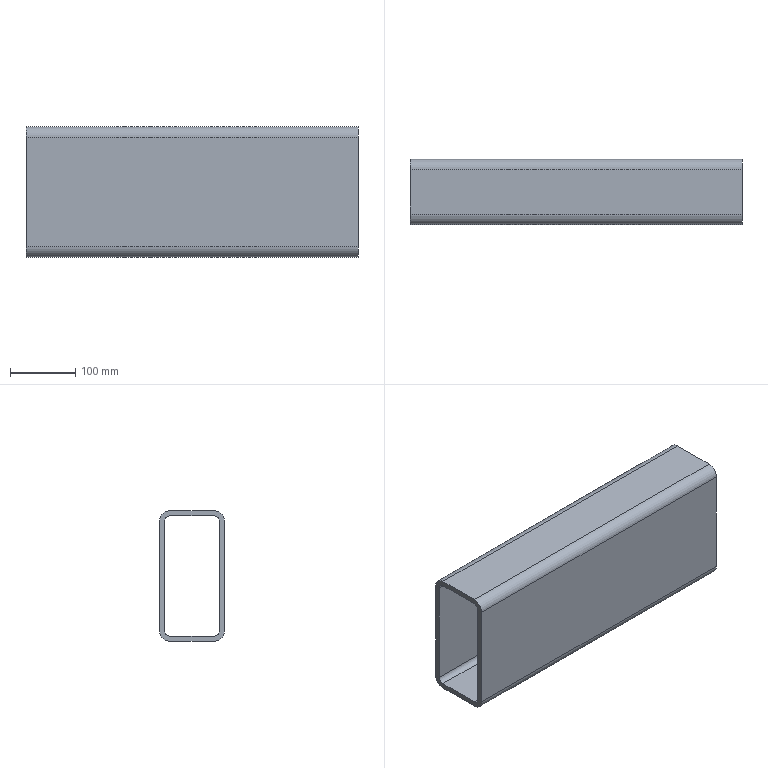Part | STEP file | 05-Longitudinal beam (flat tube 200x100x8)_default<machining> | 1 solid | 18 faces | box 509 x 100 x 200 mm | volume 2229006 mm3 | plane 10 | cylinder 8 | commonest cylinder face diameters 16 x4 32 x4
STEP:
#1=CARTESIAN_POINT('',(0.,0.,0.));
#2=DIRECTION('',(0.,0.,1.));
#3=DIRECTION('',(1.,0.,0.));
#4=AXIS2_PLACEMENT_3D('',#1,#2,#3);
#5=CARTESIAN_POINT('',(0.,50.,84.));
#6=VERTEX_POINT('',#5);
#7=CARTESIAN_POINT('',(0.,34.,100.));
#8=VERTEX_POINT('',#7);
#9=CARTESIAN_POINT('',(0.,34.,84.));
#10=DIRECTION('',(1.,0.,0.));
#11=DIRECTION('',(0.,0.,-1.));
#12=AXIS2_PLACEMENT_3D('',#9,#10,#11);
#13=CIRCLE('',#12,16.);
#14=CARTESIAN_POINT('',(509.,34.,84.));
#15=DIRECTION('',(-1.,0.,0.));
#16=DIRECTION('',(0.,0.,1.));
#17=AXIS2_PLACEMENT_3D('',#14,#15,#16);
#18=CYLINDRICAL_SURFACE('',#17,16.);
#19=CARTESIAN_POINT('',(3.142,509.));
#20=DIRECTION('',(-1.,0.));
#21=VECTOR('',#20,1.);
#22=LINE('',#19,#21);
#23=(GEOMETRIC_REPRESENTATION_CONTEXT(2)PARAMETRIC_REPRESENTATION_CONTEXT()REPRESENTATION_CONTEXT('',''));
#24=DEFINITIONAL_REPRESENTATION('',(#22),#23);
#25=PCURVE('',#18,#24);
#26=CARTESIAN_POINT('',(0.,34.,84.));
#27=DIRECTION('',(1.,0.,0.));
#28=DIRECTION('',(0.,0.,-1.));
#29=AXIS2_PLACEMENT_3D('',#26,#27,#28);
#30=PLANE('',#29);
#31=CARTESIAN_POINT('',(0.,0.));
#32=DIRECTION('',(1.,0.));
#33=AXIS2_PLACEMENT_2D('',#31,#32);
#34=CIRCLE('',#33,16.);
#35=(GEOMETRIC_REPRESENTATION_CONTEXT(2)PARAMETRIC_REPRESENTATION_CONTEXT()REPRESENTATION_CONTEXT('',''));
#36=DEFINITIONAL_REPRESENTATION('',(#34),#35);
#37=PCURVE('',#30,#36);
#38=SURFACE_CURVE('',#13,(#25,#37),.PCURVE_S1.);
#39=EDGE_CURVE('',#6,#8,#38,.T.);
#40=ORIENTED_EDGE('',*,*,#39,.T.);
#41=CARTESIAN_POINT('',(509.,34.,100.));
#42=VERTEX_POINT('',#41);
#43=CARTESIAN_POINT('',(509.,34.,100.));
#44=DIRECTION('',(-1.,0.,0.));
#45=VECTOR('',#44,1.);
#46=LINE('',#43,#45);
#47=CARTESIAN_POINT('',(0.,0.));
#48=DIRECTION('',(0.,1.));
#49=VECTOR('',#48,1.);
#50=LINE('',#47,#49);
#51=(GEOMETRIC_REPRESENTATION_CONTEXT(2)PARAMETRIC_REPRESENTATION_CONTEXT()REPRESENTATION_CONTEXT('',''));
#52=DEFINITIONAL_REPRESENTATION('',(#50),#51);
#53=PCURVE('',#18,#52);
#54=CARTESIAN_POINT('',(509.,34.,100.));
#55=DIRECTION('',(0.,0.,-1.));
#56=DIRECTION('',(-1.,0.,0.));
#57=AXIS2_PLACEMENT_3D('',#54,#55,#56);
#58=PLANE('',#57);
#59=CARTESIAN_POINT('',(0.,0.));
#60=DIRECTION('',(1.,0.));
#61=VECTOR('',#60,1.);
#62=LINE('',#59,#61);
#63=(GEOMETRIC_REPRESENTATION_CONTEXT(2)PARAMETRIC_REPRESENTATION_CONTEXT()REPRESENTATION_CONTEXT('',''));
#64=DEFINITIONAL_REPRESENTATION('',(#62),#63);
#65=PCURVE('',#58,#64);
#66=SURFACE_CURVE('',#46,(#53,#65),.PCURVE_S1.);
#67=EDGE_CURVE('',#42,#8,#66,.T.);
#68=ORIENTED_EDGE('',*,*,#67,.F.);
#69=CARTESIAN_POINT('',(509.,50.,84.));
#70=VERTEX_POINT('',#69);
#71=CARTESIAN_POINT('',(509.,34.,84.));
#72=DIRECTION('',(1.,0.,0.));
#73=DIRECTION('',(0.,0.,-1.));
#74=AXIS2_PLACEMENT_3D('',#71,#72,#73);
#75=CIRCLE('',#74,16.);
#76=CARTESIAN_POINT('',(3.142,0.));
#77=DIRECTION('',(-1.,0.));
#78=VECTOR('',#77,1.);
#79=LINE('',#76,#78);
#80=(GEOMETRIC_REPRESENTATION_CONTEXT(2)PARAMETRIC_REPRESENTATION_CONTEXT()REPRESENTATION_CONTEXT('',''));
#81=DEFINITIONAL_REPRESENTATION('',(#79),#80);
#82=PCURVE('',#18,#81);
#83=CARTESIAN_POINT('',(509.,34.,84.));
#84=DIRECTION('',(1.,0.,0.));
#85=DIRECTION('',(0.,0.,-1.));
#86=AXIS2_PLACEMENT_3D('',#83,#84,#85);
#87=PLANE('',#86);
#88=CARTESIAN_POINT('',(0.,0.));
#89=DIRECTION('',(1.,0.));
#90=AXIS2_PLACEMENT_2D('',#88,#89);
#91=CIRCLE('',#90,16.);
#92=(GEOMETRIC_REPRESENTATION_CONTEXT(2)PARAMETRIC_REPRESENTATION_CONTEXT()REPRESENTATION_CONTEXT('',''));
#93=DEFINITIONAL_REPRESENTATION('',(#91),#92);
#94=PCURVE('',#87,#93);
#95=SURFACE_CURVE('',#75,(#82,#94),.PCURVE_S1.);
#96=EDGE_CURVE('',#70,#42,#95,.T.);
#97=ORIENTED_EDGE('',*,*,#96,.F.);
#98=CARTESIAN_POINT('',(509.,50.,84.));
#99=DIRECTION('',(-1.,0.,0.));
#100=VECTOR('',#99,1.);
#101=LINE('',#98,#100);
#102=CARTESIAN_POINT('',(1.571,0.));
#103=DIRECTION('',(0.,1.));
#104=VECTOR('',#103,1.);
#105=LINE('',#102,#104);
#106=(GEOMETRIC_REPRESENTATION_CONTEXT(2)PARAMETRIC_REPRESENTATION_CONTEXT()REPRESENTATION_CONTEXT('',''));
#107=DEFINITIONAL_REPRESENTATION('',(#105),#106);
#108=PCURVE('',#18,#107);
#109=CARTESIAN_POINT('',(509.,50.,84.));
#110=DIRECTION('',(0.,-1.,0.));
#111=DIRECTION('',(0.,0.,-1.));
#112=AXIS2_PLACEMENT_3D('',#109,#110,#111);
#113=PLANE('',#112);
#114=CARTESIAN_POINT('',(0.,0.));
#115=DIRECTION('',(0.,-1.));
#116=VECTOR('',#115,1.);
#117=LINE('',#114,#116);
#118=(GEOMETRIC_REPRESENTATION_CONTEXT(2)PARAMETRIC_REPRESENTATION_CONTEXT()REPRESENTATION_CONTEXT('',''));
#119=DEFINITIONAL_REPRESENTATION('',(#117),#118);
#120=PCURVE('',#113,#119);
#121=SURFACE_CURVE('',#101,(#108,#120),.PCURVE_S1.);
#122=EDGE_CURVE('',#70,#6,#121,.T.);
#123=ORIENTED_EDGE('',*,*,#122,.T.);
#124=EDGE_LOOP('',(#40,#68,#97,#123));
#125=FACE_BOUND('',#124,.T.);
#126=ADVANCED_FACE('',(#125),#18,.T.);
#127=CARTESIAN_POINT('',(0.,-34.,100.));
#128=VERTEX_POINT('',#127);
#129=CARTESIAN_POINT('',(0.,34.,100.));
#130=DIRECTION('',(0.,-1.,0.));
#131=VECTOR('',#130,1.);
#132=LINE('',#129,#131);
#133=CARTESIAN_POINT('',(509.,0.));
#134=DIRECTION('',(0.,-1.));
#135=VECTOR('',#134,1.);
#136=LINE('',#133,#135);
#137=(GEOMETRIC_REPRESENTATION_CONTEXT(2)PARAMETRIC_REPRESENTATION_CONTEXT()REPRESENTATION_CONTEXT('',''));
#138=DEFINITIONAL_REPRESENTATION('',(#136),#137);
#139=PCURVE('',#58,#138);
#140=CARTESIAN_POINT('',(-16.,0.));
#141=DIRECTION('',(0.,-1.));
#142=VECTOR('',#141,1.);
#143=LINE('',#140,#142);
#144=(GEOMETRIC_REPRESENTATION_CONTEXT(2)PARAMETRIC_REPRESENTATION_CONTEXT()REPRESENTATION_CONTEXT('',''));
#145=DEFINITIONAL_REPRESENTATION('',(#143),#144);
#146=PCURVE('',#30,#145);
#147=SURFACE_CURVE('',#132,(#139,#146),.PCURVE_S1.);
#148=EDGE_CURVE('',#8,#128,#147,.T.);
#149=ORIENTED_EDGE('',*,*,#148,.T.);
#150=CARTESIAN_POINT('',(509.,-34.,100.));
#151=VERTEX_POINT('',#150);
#152=CARTESIAN_POINT('',(509.,-34.,100.));
#153=DIRECTION('',(-1.,0.,0.));
#154=VECTOR('',#153,1.);
#155=LINE('',#152,#154);
#156=CARTESIAN_POINT('',(0.,-68.));
#157=DIRECTION('',(1.,0.));
#158=VECTOR('',#157,1.);
#159=LINE('',#156,#158);
#160=(GEOMETRIC_REPRESENTATION_CONTEXT(2)PARAMETRIC_REPRESENTATION_CONTEXT()REPRESENTATION_CONTEXT('',''));
#161=DEFINITIONAL_REPRESENTATION('',(#159),#160);
#162=PCURVE('',#58,#161);
#163=CARTESIAN_POINT('',(509.,-34.,84.));
#164=DIRECTION('',(-1.,0.,0.));
#165=DIRECTION('',(0.,0.,1.));
#166=AXIS2_PLACEMENT_3D('',#163,#164,#165);
#167=CYLINDRICAL_SURFACE('',#166,16.);
#168=CARTESIAN_POINT('',(6.283,0.));
#169=DIRECTION('',(0.,1.));
#170=VECTOR('',#169,1.);
#171=LINE('',#168,#170);
#172=(GEOMETRIC_REPRESENTATION_CONTEXT(2)PARAMETRIC_REPRESENTATION_CONTEXT()REPRESENTATION_CONTEXT('',''));
#173=DEFINITIONAL_REPRESENTATION('',(#171),#172);
#174=PCURVE('',#167,#173);
#175=SURFACE_CURVE('',#155,(#162,#174),.PCURVE_S1.);
#176=EDGE_CURVE('',#151,#128,#175,.T.);
#177=ORIENTED_EDGE('',*,*,#176,.F.);
#178=CARTESIAN_POINT('',(509.,34.,100.));
#179=DIRECTION('',(0.,-1.,0.));
#180=VECTOR('',#179,1.);
#181=LINE('',#178,#180);
#182=CARTESIAN_POINT('',(0.,0.));
#183=DIRECTION('',(0.,-1.));
#184=VECTOR('',#183,1.);
#185=LINE('',#182,#184);
#186=(GEOMETRIC_REPRESENTATION_CONTEXT(2)PARAMETRIC_REPRESENTATION_CONTEXT()REPRESENTATION_CONTEXT('',''));
#187=DEFINITIONAL_REPRESENTATION('',(#185),#186);
#188=PCURVE('',#58,#187);
#189=CARTESIAN_POINT('',(-16.,0.));
#190=DIRECTION('',(0.,-1.));
#191=VECTOR('',#190,1.);
#192=LINE('',#189,#191);
#193=(GEOMETRIC_REPRESENTATION_CONTEXT(2)PARAMETRIC_REPRESENTATION_CONTEXT()REPRESENTATION_CONTEXT('',''));
#194=DEFINITIONAL_REPRESENTATION('',(#192),#193);
#195=PCURVE('',#87,#194);
#196=SURFACE_CURVE('',#181,(#188,#195),.PCURVE_S1.);
#197=EDGE_CURVE('',#42,#151,#196,.T.);
#198=ORIENTED_EDGE('',*,*,#197,.F.);
#199=ORIENTED_EDGE('',*,*,#67,.T.);
#200=EDGE_LOOP('',(#149,#177,#198,#199));
#201=FACE_BOUND('',#200,.T.);
#202=ADVANCED_FACE('',(#201),#58,.F.);
#203=CARTESIAN_POINT('',(0.,-50.,84.));
#204=VERTEX_POINT('',#203);
#205=CARTESIAN_POINT('',(0.,-34.,84.));
#206=DIRECTION('',(1.,0.,0.));
#207=DIRECTION('',(0.,0.,-1.));
#208=AXIS2_PLACEMENT_3D('',#205,#206,#207);
#209=CIRCLE('',#208,16.);
#210=CARTESIAN_POINT('',(9.425,509.));
#211=DIRECTION('',(-1.,0.));
#212=VECTOR('',#211,1.);
#213=LINE('',#210,#212);
#214=(GEOMETRIC_REPRESENTATION_CONTEXT(2)PARAMETRIC_REPRESENTATION_CONTEXT()REPRESENTATION_CONTEXT('',''));
#215=DEFINITIONAL_REPRESENTATION('',(#213),#214);
#216=PCURVE('',#167,#215);
#217=CARTESIAN_POINT('',(0.,-68.));
#218=DIRECTION('',(1.,0.));
#219=AXIS2_PLACEMENT_2D('',#217,#218);
#220=CIRCLE('',#219,16.);
#221=(GEOMETRIC_REPRESENTATION_CONTEXT(2)PARAMETRIC_REPRESENTATION_CONTEXT()REPRESENTATION_CONTEXT('',''));
#222=DEFINITIONAL_REPRESENTATION('',(#220),#221);
#223=PCURVE('',#30,#222);
#224=SURFACE_CURVE('',#209,(#216,#223),.PCURVE_S1.);
#225=EDGE_CURVE('',#128,#204,#224,.T.);
#226=ORIENTED_EDGE('',*,*,#225,.T.);
#227=CARTESIAN_POINT('',(509.,-50.,84.));
#228=VERTEX_POINT('',#227);
#229=CARTESIAN_POINT('',(509.,-50.,84.));
#230=DIRECTION('',(-1.,0.,0.));
#231=VECTOR('',#230,1.);
#232=LINE('',#229,#231);
#233=CARTESIAN_POINT('',(4.712,0.));
#234=DIRECTION('',(0.,1.));
#235=VECTOR('',#234,1.);
#236=LINE('',#233,#235);
#237=(GEOMETRIC_REPRESENTATION_CONTEXT(2)PARAMETRIC_REPRESENTATION_CONTEXT()REPRESENTATION_CONTEXT('',''));
#238=DEFINITIONAL_REPRESENTATION('',(#236),#237);
#239=PCURVE('',#167,#238);
#240=CARTESIAN_POINT('',(509.,-50.,-84.));
#241=DIRECTION('',(0.,1.,0.));
#242=DIRECTION('',(0.,0.,1.));
#243=AXIS2_PLACEMENT_3D('',#240,#241,#242);
#244=PLANE('',#243);
#245=CARTESIAN_POINT('',(168.,0.));
#246=DIRECTION('',(0.,-1.));
#247=VECTOR('',#246,1.);
#248=LINE('',#245,#247);
#249=(GEOMETRIC_REPRESENTATION_CONTEXT(2)PARAMETRIC_REPRESENTATION_CONTEXT()REPRESENTATION_CONTEXT('',''));
#250=DEFINITIONAL_REPRESENTATION('',(#248),#249);
#251=PCURVE('',#244,#250);
#252=SURFACE_CURVE('',#232,(#239,#251),.PCURVE_S1.);
#253=EDGE_CURVE('',#228,#204,#252,.T.);
#254=ORIENTED_EDGE('',*,*,#253,.F.);
#255=CARTESIAN_POINT('',(509.,-34.,84.));
#256=DIRECTION('',(1.,0.,0.));
#257=DIRECTION('',(0.,0.,-1.));
#258=AXIS2_PLACEMENT_3D('',#255,#256,#257);
#259=CIRCLE('',#258,16.);
#260=CARTESIAN_POINT('',(9.425,0.));
#261=DIRECTION('',(-1.,0.));
#262=VECTOR('',#261,1.);
#263=LINE('',#260,#262);
#264=(GEOMETRIC_REPRESENTATION_CONTEXT(2)PARAMETRIC_REPRESENTATION_CONTEXT()REPRESENTATION_CONTEXT('',''));
#265=DEFINITIONAL_REPRESENTATION('',(#263),#264);
#266=PCURVE('',#167,#265);
#267=CARTESIAN_POINT('',(0.,-68.));
#268=DIRECTION('',(1.,0.));
#269=AXIS2_PLACEMENT_2D('',#267,#268);
#270=CIRCLE('',#269,16.);
#271=(GEOMETRIC_REPRESENTATION_CONTEXT(2)PARAMETRIC_REPRESENTATION_CONTEXT()REPRESENTATION_CONTEXT('',''));
#272=DEFINITIONAL_REPRESENTATION('',(#270),#271);
#273=PCURVE('',#87,#272);
#274=SURFACE_CURVE('',#259,(#266,#273),.PCURVE_S1.);
#275=EDGE_CURVE('',#151,#228,#274,.T.);
#276=ORIENTED_EDGE('',*,*,#275,.F.);
#277=ORIENTED_EDGE('',*,*,#176,.T.);
#278=EDGE_LOOP('',(#226,#254,#276,#277));
#279=FACE_BOUND('',#278,.T.);
#280=ADVANCED_FACE('',(#279),#167,.T.);
#281=CARTESIAN_POINT('',(0.,-50.,-84.));
#282=VERTEX_POINT('',#281);
#283=CARTESIAN_POINT('',(0.,-50.,-84.));
#284=DIRECTION('',(0.,0.,-1.));
#285=VECTOR('',#284,1.);
#286=LINE('',#283,#285);
#287=CARTESIAN_POINT('',(0.,-509.));
#288=DIRECTION('',(-1.,0.));
#289=VECTOR('',#288,1.);
#290=LINE('',#287,#289);
#291=(GEOMETRIC_REPRESENTATION_CONTEXT(2)PARAMETRIC_REPRESENTATION_CONTEXT()REPRESENTATION_CONTEXT('',''));
#292=DEFINITIONAL_REPRESENTATION('',(#290),#291);
#293=PCURVE('',#244,#292);
#294=CARTESIAN_POINT('',(168.,-84.));
#295=DIRECTION('',(1.,0.));
#296=VECTOR('',#295,1.);
#297=LINE('',#294,#296);
#298=(GEOMETRIC_REPRESENTATION_CONTEXT(2)PARAMETRIC_REPRESENTATION_CONTEXT()REPRESENTATION_CONTEXT('',''));
#299=DEFINITIONAL_REPRESENTATION('',(#297),#298);
#300=PCURVE('',#30,#299);
#301=SURFACE_CURVE('',#286,(#293,#300),.PCURVE_S1.);
#302=EDGE_CURVE('',#204,#282,#301,.T.);
#303=ORIENTED_EDGE('',*,*,#302,.T.);
#304=CARTESIAN_POINT('',(509.,-50.,-84.));
#305=VERTEX_POINT('',#304);
#306=CARTESIAN_POINT('',(509.,-50.,-84.));
#307=DIRECTION('',(-1.,0.,0.));
#308=VECTOR('',#307,1.);
#309=LINE('',#306,#308);
#310=CARTESIAN_POINT('',(0.,0.));
#311=DIRECTION('',(0.,-1.));
#312=VECTOR('',#311,1.);
#313=LINE('',#310,#312);
#314=(GEOMETRIC_REPRESENTATION_CONTEXT(2)PARAMETRIC_REPRESENTATION_CONTEXT()REPRESENTATION_CONTEXT('',''));
#315=DEFINITIONAL_REPRESENTATION('',(#313),#314);
#316=PCURVE('',#244,#315);
#317=CARTESIAN_POINT('',(509.,-34.,-84.));
#318=DIRECTION('',(-1.,0.,0.));
#319=DIRECTION('',(0.,0.,1.));
#320=AXIS2_PLACEMENT_3D('',#317,#318,#319);
#321=CYLINDRICAL_SURFACE('',#320,16.);
#322=CARTESIAN_POINT('',(4.712,0.));
#323=DIRECTION('',(0.,1.));
#324=VECTOR('',#323,1.);
#325=LINE('',#322,#324);
#326=(GEOMETRIC_REPRESENTATION_CONTEXT(2)PARAMETRIC_REPRESENTATION_CONTEXT()REPRESENTATION_CONTEXT('',''));
#327=DEFINITIONAL_REPRESENTATION('',(#325),#326);
#328=PCURVE('',#321,#327);
#329=SURFACE_CURVE('',#309,(#316,#328),.PCURVE_S1.);
#330=EDGE_CURVE('',#305,#282,#329,.T.);
#331=ORIENTED_EDGE('',*,*,#330,.F.);
#332=CARTESIAN_POINT('',(509.,-50.,-84.));
#333=DIRECTION('',(0.,0.,-1.));
#334=VECTOR('',#333,1.);
#335=LINE('',#332,#334);
#336=CARTESIAN_POINT('',(0.,0.));
#337=DIRECTION('',(-1.,0.));
#338=VECTOR('',#337,1.);
#339=LINE('',#336,#338);
#340=(GEOMETRIC_REPRESENTATION_CONTEXT(2)PARAMETRIC_REPRESENTATION_CONTEXT()REPRESENTATION_CONTEXT('',''));
#341=DEFINITIONAL_REPRESENTATION('',(#339),#340);
#342=PCURVE('',#244,#341);
#343=CARTESIAN_POINT('',(168.,-84.));
#344=DIRECTION('',(1.,0.));
#345=VECTOR('',#344,1.);
#346=LINE('',#343,#345);
#347=(GEOMETRIC_REPRESENTATION_CONTEXT(2)PARAMETRIC_REPRESENTATION_CONTEXT()REPRESENTATION_CONTEXT('',''));
#348=DEFINITIONAL_REPRESENTATION('',(#346),#347);
#349=PCURVE('',#87,#348);
#350=SURFACE_CURVE('',#335,(#342,#349),.PCURVE_S1.);
#351=EDGE_CURVE('',#228,#305,#350,.T.);
#352=ORIENTED_EDGE('',*,*,#351,.F.);
#353=ORIENTED_EDGE('',*,*,#253,.T.);
#354=EDGE_LOOP('',(#303,#331,#352,#353));
#355=FACE_BOUND('',#354,.T.);
#356=ADVANCED_FACE('',(#355),#244,.F.);
#357=CARTESIAN_POINT('',(0.,-34.,-100.));
#358=VERTEX_POINT('',#357);
#359=CARTESIAN_POINT('',(0.,-34.,-84.));
#360=DIRECTION('',(1.,0.,0.));
#361=DIRECTION('',(0.,0.,-1.));
#362=AXIS2_PLACEMENT_3D('',#359,#360,#361);
#363=CIRCLE('',#362,16.);
#364=CARTESIAN_POINT('',(9.425,509.));
#365=DIRECTION('',(-1.,0.));
#366=VECTOR('',#365,1.);
#367=LINE('',#364,#366);
#368=(GEOMETRIC_REPRESENTATION_CONTEXT(2)PARAMETRIC_REPRESENTATION_CONTEXT()REPRESENTATION_CONTEXT('',''));
#369=DEFINITIONAL_REPRESENTATION('',(#367),#368);
#370=PCURVE('',#321,#369);
#371=CARTESIAN_POINT('',(168.,-68.));
#372=DIRECTION('',(1.,0.));
#373=AXIS2_PLACEMENT_2D('',#371,#372);
#374=CIRCLE('',#373,16.);
#375=(GEOMETRIC_REPRESENTATION_CONTEXT(2)PARAMETRIC_REPRESENTATION_CONTEXT()REPRESENTATION_CONTEXT('',''));
#376=DEFINITIONAL_REPRESENTATION('',(#374),#375);
#377=PCURVE('',#30,#376);
#378=SURFACE_CURVE('',#363,(#370,#377),.PCURVE_S1.);
#379=EDGE_CURVE('',#282,#358,#378,.T.);
#380=ORIENTED_EDGE('',*,*,#379,.T.);
#381=CARTESIAN_POINT('',(509.,-34.,-100.));
#382=VERTEX_POINT('',#381);
#383=CARTESIAN_POINT('',(509.,-34.,-100.));
#384=DIRECTION('',(-1.,0.,0.));
#385=VECTOR('',#384,1.);
#386=LINE('',#383,#385);
#387=CARTESIAN_POINT('',(3.142,0.));
#388=DIRECTION('',(0.,1.));
#389=VECTOR('',#388,1.);
#390=LINE('',#387,#389);
#391=(GEOMETRIC_REPRESENTATION_CONTEXT(2)PARAMETRIC_REPRESENTATION_CONTEXT()REPRESENTATION_CONTEXT('',''));
#392=DEFINITIONAL_REPRESENTATION('',(#390),#391);
#393=PCURVE('',#321,#392);
#394=CARTESIAN_POINT('',(509.,-34.,-100.));
#395=DIRECTION('',(0.,0.,1.));
#396=DIRECTION('',(1.,0.,0.));
#397=AXIS2_PLACEMENT_3D('',#394,#395,#396);
#398=PLANE('',#397);
#399=CARTESIAN_POINT('',(0.,0.));
#400=DIRECTION('',(-1.,0.));
#401=VECTOR('',#400,1.);
#402=LINE('',#399,#401);
#403=(GEOMETRIC_REPRESENTATION_CONTEXT(2)PARAMETRIC_REPRESENTATION_CONTEXT()REPRESENTATION_CONTEXT('',''));
#404=DEFINITIONAL_REPRESENTATION('',(#402),#403);
#405=PCURVE('',#398,#404);
#406=SURFACE_CURVE('',#386,(#393,#405),.PCURVE_S1.);
#407=EDGE_CURVE('',#382,#358,#406,.T.);
#408=ORIENTED_EDGE('',*,*,#407,.F.);
#409=CARTESIAN_POINT('',(509.,-34.,-84.));
#410=DIRECTION('',(1.,0.,0.));
#411=DIRECTION('',(0.,0.,-1.));
#412=AXIS2_PLACEMENT_3D('',#409,#410,#411);
#413=CIRCLE('',#412,16.);
#414=CARTESIAN_POINT('',(9.425,0.));
#415=DIRECTION('',(-1.,0.));
#416=VECTOR('',#415,1.);
#417=LINE('',#414,#416);
#418=(GEOMETRIC_REPRESENTATION_CONTEXT(2)PARAMETRIC_REPRESENTATION_CONTEXT()REPRESENTATION_CONTEXT('',''));
#419=DEFINITIONAL_REPRESENTATION('',(#417),#418);
#420=PCURVE('',#321,#419);
#421=CARTESIAN_POINT('',(168.,-68.));
#422=DIRECTION('',(1.,0.));
#423=AXIS2_PLACEMENT_2D('',#421,#422);
#424=CIRCLE('',#423,16.);
#425=(GEOMETRIC_REPRESENTATION_CONTEXT(2)PARAMETRIC_REPRESENTATION_CONTEXT()REPRESENTATION_CONTEXT('',''));
#426=DEFINITIONAL_REPRESENTATION('',(#424),#425);
#427=PCURVE('',#87,#426);
#428=SURFACE_CURVE('',#413,(#420,#427),.PCURVE_S1.);
#429=EDGE_CURVE('',#305,#382,#428,.T.);
#430=ORIENTED_EDGE('',*,*,#429,.F.);
#431=ORIENTED_EDGE('',*,*,#330,.T.);
#432=EDGE_LOOP('',(#380,#408,#430,#431));
#433=FACE_BOUND('',#432,.T.);
#434=ADVANCED_FACE('',(#433),#321,.T.);
#435=CARTESIAN_POINT('',(0.,34.,-100.));
#436=VERTEX_POINT('',#435);
#437=CARTESIAN_POINT('',(0.,-34.,-100.));
#438=DIRECTION('',(0.,1.,0.));
#439=VECTOR('',#438,1.);
#440=LINE('',#437,#439);
#441=CARTESIAN_POINT('',(-509.,0.));
#442=DIRECTION('',(0.,1.));
#443=VECTOR('',#442,1.);
#444=LINE('',#441,#443);
#445=(GEOMETRIC_REPRESENTATION_CONTEXT(2)PARAMETRIC_REPRESENTATION_CONTEXT()REPRESENTATION_CONTEXT('',''));
#446=DEFINITIONAL_REPRESENTATION('',(#444),#445);
#447=PCURVE('',#398,#446);
#448=CARTESIAN_POINT('',(184.,-68.));
#449=DIRECTION('',(0.,1.));
#450=VECTOR('',#449,1.);
#451=LINE('',#448,#450);
#452=(GEOMETRIC_REPRESENTATION_CONTEXT(2)PARAMETRIC_REPRESENTATION_CONTEXT()REPRESENTATION_CONTEXT('',''));
#453=DEFINITIONAL_REPRESENTATION('',(#451),#452);
#454=PCURVE('',#30,#453);
#455=SURFACE_CURVE('',#440,(#447,#454),.PCURVE_S1.);
#456=EDGE_CURVE('',#358,#436,#455,.T.);
#457=ORIENTED_EDGE('',*,*,#456,.T.);
#458=CARTESIAN_POINT('',(509.,34.,-100.));
#459=VERTEX_POINT('',#458);
#460=CARTESIAN_POINT('',(509.,34.,-100.));
#461=DIRECTION('',(-1.,0.,0.));
#462=VECTOR('',#461,1.);
#463=LINE('',#460,#462);
#464=CARTESIAN_POINT('',(0.,68.));
#465=DIRECTION('',(-1.,0.));
#466=VECTOR('',#465,1.);
#467=LINE('',#464,#466);
#468=(GEOMETRIC_REPRESENTATION_CONTEXT(2)PARAMETRIC_REPRESENTATION_CONTEXT()REPRESENTATION_CONTEXT('',''));
#469=DEFINITIONAL_REPRESENTATION('',(#467),#468);
#470=PCURVE('',#398,#469);
#471=CARTESIAN_POINT('',(509.,34.,-84.));
#472=DIRECTION('',(-1.,0.,0.));
#473=DIRECTION('',(0.,0.,1.));
#474=AXIS2_PLACEMENT_3D('',#471,#472,#473);
#475=CYLINDRICAL_SURFACE('',#474,16.);
#476=CARTESIAN_POINT('',(3.142,0.));
#477=DIRECTION('',(0.,1.));
#478=VECTOR('',#477,1.);
#479=LINE('',#476,#478);
#480=(GEOMETRIC_REPRESENTATION_CONTEXT(2)PARAMETRIC_REPRESENTATION_CONTEXT()REPRESENTATION_CONTEXT('',''));
#481=DEFINITIONAL_REPRESENTATION('',(#479),#480);
#482=PCURVE('',#475,#481);
#483=SURFACE_CURVE('',#463,(#470,#482),.PCURVE_S1.);
#484=EDGE_CURVE('',#459,#436,#483,.T.);
#485=ORIENTED_EDGE('',*,*,#484,.F.);
#486=CARTESIAN_POINT('',(509.,-34.,-100.));
#487=DIRECTION('',(0.,1.,0.));
#488=VECTOR('',#487,1.);
#489=LINE('',#486,#488);
#490=CARTESIAN_POINT('',(0.,0.));
#491=DIRECTION('',(0.,1.));
#492=VECTOR('',#491,1.);
#493=LINE('',#490,#492);
#494=(GEOMETRIC_REPRESENTATION_CONTEXT(2)PARAMETRIC_REPRESENTATION_CONTEXT()REPRESENTATION_CONTEXT('',''));
#495=DEFINITIONAL_REPRESENTATION('',(#493),#494);
#496=PCURVE('',#398,#495);
#497=CARTESIAN_POINT('',(184.,-68.));
#498=DIRECTION('',(0.,1.));
#499=VECTOR('',#498,1.);
#500=LINE('',#497,#499);
#501=(GEOMETRIC_REPRESENTATION_CONTEXT(2)PARAMETRIC_REPRESENTATION_CONTEXT()REPRESENTATION_CONTEXT('',''));
#502=DEFINITIONAL_REPRESENTATION('',(#500),#501);
#503=PCURVE('',#87,#502);
#504=SURFACE_CURVE('',#489,(#496,#503),.PCURVE_S1.);
#505=EDGE_CURVE('',#382,#459,#504,.T.);
#506=ORIENTED_EDGE('',*,*,#505,.F.);
#507=ORIENTED_EDGE('',*,*,#407,.T.);
#508=EDGE_LOOP('',(#457,#485,#506,#507));
#509=FACE_BOUND('',#508,.T.);
#510=ADVANCED_FACE('',(#509),#398,.F.);
#511=CARTESIAN_POINT('',(0.,50.,-84.));
#512=VERTEX_POINT('',#511);
#513=CARTESIAN_POINT('',(0.,34.,-84.));
#514=DIRECTION('',(1.,0.,0.));
#515=DIRECTION('',(0.,0.,-1.));
#516=AXIS2_PLACEMENT_3D('',#513,#514,#515);
#517=CIRCLE('',#516,16.);
#518=CARTESIAN_POINT('',(3.142,509.));
#519=DIRECTION('',(-1.,0.));
#520=VECTOR('',#519,1.);
#521=LINE('',#518,#520);
#522=(GEOMETRIC_REPRESENTATION_CONTEXT(2)PARAMETRIC_REPRESENTATION_CONTEXT()REPRESENTATION_CONTEXT('',''));
#523=DEFINITIONAL_REPRESENTATION('',(#521),#522);
#524=PCURVE('',#475,#523);
#525=CARTESIAN_POINT('',(168.,0.));
#526=DIRECTION('',(1.,0.));
#527=AXIS2_PLACEMENT_2D('',#525,#526);
#528=CIRCLE('',#527,16.);
#529=(GEOMETRIC_REPRESENTATION_CONTEXT(2)PARAMETRIC_REPRESENTATION_CONTEXT()REPRESENTATION_CONTEXT('',''));
#530=DEFINITIONAL_REPRESENTATION('',(#528),#529);
#531=PCURVE('',#30,#530);
#532=SURFACE_CURVE('',#517,(#524,#531),.PCURVE_S1.);
#533=EDGE_CURVE('',#436,#512,#532,.T.);
#534=ORIENTED_EDGE('',*,*,#533,.T.);
#535=CARTESIAN_POINT('',(509.,50.,-84.));
#536=VERTEX_POINT('',#535);
#537=CARTESIAN_POINT('',(509.,50.,-84.));
#538=DIRECTION('',(-1.,0.,0.));
#539=VECTOR('',#538,1.);
#540=LINE('',#537,#539);
#541=CARTESIAN_POINT('',(1.571,0.));
#542=DIRECTION('',(0.,1.));
#543=VECTOR('',#542,1.);
#544=LINE('',#541,#543);
#545=(GEOMETRIC_REPRESENTATION_CONTEXT(2)PARAMETRIC_REPRESENTATION_CONTEXT()REPRESENTATION_CONTEXT('',''));
#546=DEFINITIONAL_REPRESENTATION('',(#544),#545);
#547=PCURVE('',#475,#546);
#548=CARTESIAN_POINT('',(168.,0.));
#549=DIRECTION('',(0.,-1.));
#550=VECTOR('',#549,1.);
#551=LINE('',#548,#550);
#552=(GEOMETRIC_REPRESENTATION_CONTEXT(2)PARAMETRIC_REPRESENTATION_CONTEXT()REPRESENTATION_CONTEXT('',''));
#553=DEFINITIONAL_REPRESENTATION('',(#551),#552);
#554=PCURVE('',#113,#553);
#555=SURFACE_CURVE('',#540,(#547,#554),.PCURVE_S1.);
#556=EDGE_CURVE('',#536,#512,#555,.T.);
#557=ORIENTED_EDGE('',*,*,#556,.F.);
#558=CARTESIAN_POINT('',(509.,34.,-84.));
#559=DIRECTION('',(1.,0.,0.));
#560=DIRECTION('',(0.,0.,-1.));
#561=AXIS2_PLACEMENT_3D('',#558,#559,#560);
#562=CIRCLE('',#561,16.);
#563=CARTESIAN_POINT('',(3.142,0.));
#564=DIRECTION('',(-1.,0.));
#565=VECTOR('',#564,1.);
#566=LINE('',#563,#565);
#567=(GEOMETRIC_REPRESENTATION_CONTEXT(2)PARAMETRIC_REPRESENTATION_CONTEXT()REPRESENTATION_CONTEXT('',''));
#568=DEFINITIONAL_REPRESENTATION('',(#566),#567);
#569=PCURVE('',#475,#568);
#570=CARTESIAN_POINT('',(168.,0.));
#571=DIRECTION('',(1.,0.));
#572=AXIS2_PLACEMENT_2D('',#570,#571);
#573=CIRCLE('',#572,16.);
#574=(GEOMETRIC_REPRESENTATION_CONTEXT(2)PARAMETRIC_REPRESENTATION_CONTEXT()REPRESENTATION_CONTEXT('',''));
#575=DEFINITIONAL_REPRESENTATION('',(#573),#574);
#576=PCURVE('',#87,#575);
#577=SURFACE_CURVE('',#562,(#569,#576),.PCURVE_S1.);
#578=EDGE_CURVE('',#459,#536,#577,.T.);
#579=ORIENTED_EDGE('',*,*,#578,.F.);
#580=ORIENTED_EDGE('',*,*,#484,.T.);
#581=EDGE_LOOP('',(#534,#557,#579,#580));
#582=FACE_BOUND('',#581,.T.);
#583=ADVANCED_FACE('',(#582),#475,.T.);
#584=CARTESIAN_POINT('',(509.,-42.,84.));
#585=VERTEX_POINT('',#584);
#586=CARTESIAN_POINT('',(0.,-42.,84.));
#587=VERTEX_POINT('',#586);
#588=CARTESIAN_POINT('',(509.,-42.,84.));
#589=DIRECTION('',(-1.,0.,0.));
#590=VECTOR('',#589,1.);
#591=LINE('',#588,#590);
#592=CARTESIAN_POINT('',(509.,-34.,84.));
#593=DIRECTION('',(-1.,0.,0.));
#594=DIRECTION('',(0.,0.,1.));
#595=AXIS2_PLACEMENT_3D('',#592,#593,#594);
#596=CYLINDRICAL_SURFACE('',#595,8.);
#597=CARTESIAN_POINT('',(4.712,0.));
#598=DIRECTION('',(0.,1.));
#599=VECTOR('',#598,1.);
#600=LINE('',#597,#599);
#601=(GEOMETRIC_REPRESENTATION_CONTEXT(2)PARAMETRIC_REPRESENTATION_CONTEXT()REPRESENTATION_CONTEXT('',''));
#602=DEFINITIONAL_REPRESENTATION('',(#600),#601);
#603=PCURVE('',#596,#602);
#604=CARTESIAN_POINT('',(509.,-42.,-84.));
#605=DIRECTION('',(0.,1.,0.));
#606=DIRECTION('',(0.,0.,1.));
#607=AXIS2_PLACEMENT_3D('',#604,#605,#606);
#608=PLANE('',#607);
#609=CARTESIAN_POINT('',(168.,0.));
#610=DIRECTION('',(0.,-1.));
#611=VECTOR('',#610,1.);
#612=LINE('',#609,#611);
#613=(GEOMETRIC_REPRESENTATION_CONTEXT(2)PARAMETRIC_REPRESENTATION_CONTEXT()REPRESENTATION_CONTEXT('',''));
#614=DEFINITIONAL_REPRESENTATION('',(#612),#613);
#615=PCURVE('',#608,#614);
#616=SURFACE_CURVE('',#591,(#603,#615),.PCURVE_S1.);
#617=EDGE_CURVE('',#585,#587,#616,.T.);
#618=ORIENTED_EDGE('',*,*,#617,.F.);
#619=CARTESIAN_POINT('',(509.,-34.,92.));
#620=VERTEX_POINT('',#619);
#621=CARTESIAN_POINT('',(509.,-34.,84.));
#622=DIRECTION('',(1.,0.,0.));
#623=DIRECTION('',(0.,0.,-1.));
#624=AXIS2_PLACEMENT_3D('',#621,#622,#623);
#625=CIRCLE('',#624,8.);
#626=CARTESIAN_POINT('',(9.425,0.));
#627=DIRECTION('',(-1.,0.));
#628=VECTOR('',#627,1.);
#629=LINE('',#626,#628);
#630=(GEOMETRIC_REPRESENTATION_CONTEXT(2)PARAMETRIC_REPRESENTATION_CONTEXT()REPRESENTATION_CONTEXT('',''));
#631=DEFINITIONAL_REPRESENTATION('',(#629),#630);
#632=PCURVE('',#596,#631);
#633=CARTESIAN_POINT('',(0.,-68.));
#634=DIRECTION('',(1.,0.));
#635=AXIS2_PLACEMENT_2D('',#633,#634);
#636=CIRCLE('',#635,8.);
#637=(GEOMETRIC_REPRESENTATION_CONTEXT(2)PARAMETRIC_REPRESENTATION_CONTEXT()REPRESENTATION_CONTEXT('',''));
#638=DEFINITIONAL_REPRESENTATION('',(#636),#637);
#639=PCURVE('',#87,#638);
#640=SURFACE_CURVE('',#625,(#632,#639),.PCURVE_S1.);
#641=EDGE_CURVE('',#620,#585,#640,.T.);
#642=ORIENTED_EDGE('',*,*,#641,.F.);
#643=CARTESIAN_POINT('',(0.,-34.,92.));
#644=VERTEX_POINT('',#643);
#645=CARTESIAN_POINT('',(509.,-34.,92.));
#646=DIRECTION('',(-1.,0.,0.));
#647=VECTOR('',#646,1.);
#648=LINE('',#645,#647);
#649=CARTESIAN_POINT('',(6.283,0.));
#650=DIRECTION('',(0.,1.));
#651=VECTOR('',#650,1.);
#652=LINE('',#649,#651);
#653=(GEOMETRIC_REPRESENTATION_CONTEXT(2)PARAMETRIC_REPRESENTATION_CONTEXT()REPRESENTATION_CONTEXT('',''));
#654=DEFINITIONAL_REPRESENTATION('',(#652),#653);
#655=PCURVE('',#596,#654);
#656=CARTESIAN_POINT('',(509.,34.,92.));
#657=DIRECTION('',(0.,0.,-1.));
#658=DIRECTION('',(-1.,0.,0.));
#659=AXIS2_PLACEMENT_3D('',#656,#657,#658);
#660=PLANE('',#659);
#661=CARTESIAN_POINT('',(0.,-68.));
#662=DIRECTION('',(1.,0.));
#663=VECTOR('',#662,1.);
#664=LINE('',#661,#663);
#665=(GEOMETRIC_REPRESENTATION_CONTEXT(2)PARAMETRIC_REPRESENTATION_CONTEXT()REPRESENTATION_CONTEXT('',''));
#666=DEFINITIONAL_REPRESENTATION('',(#664),#665);
#667=PCURVE('',#660,#666);
#668=SURFACE_CURVE('',#648,(#655,#667),.PCURVE_S1.);
#669=EDGE_CURVE('',#620,#644,#668,.T.);
#670=ORIENTED_EDGE('',*,*,#669,.T.);
#671=CARTESIAN_POINT('',(0.,-34.,84.));
#672=DIRECTION('',(1.,0.,0.));
#673=DIRECTION('',(0.,0.,-1.));
#674=AXIS2_PLACEMENT_3D('',#671,#672,#673);
#675=CIRCLE('',#674,8.);
#676=CARTESIAN_POINT('',(9.425,509.));
#677=DIRECTION('',(-1.,0.));
#678=VECTOR('',#677,1.);
#679=LINE('',#676,#678);
#680=(GEOMETRIC_REPRESENTATION_CONTEXT(2)PARAMETRIC_REPRESENTATION_CONTEXT()REPRESENTATION_CONTEXT('',''));
#681=DEFINITIONAL_REPRESENTATION('',(#679),#680);
#682=PCURVE('',#596,#681);
#683=CARTESIAN_POINT('',(0.,-68.));
#684=DIRECTION('',(1.,0.));
#685=AXIS2_PLACEMENT_2D('',#683,#684);
#686=CIRCLE('',#685,8.);
#687=(GEOMETRIC_REPRESENTATION_CONTEXT(2)PARAMETRIC_REPRESENTATION_CONTEXT()REPRESENTATION_CONTEXT('',''));
#688=DEFINITIONAL_REPRESENTATION('',(#686),#687);
#689=PCURVE('',#30,#688);
#690=SURFACE_CURVE('',#675,(#682,#689),.PCURVE_S1.);
#691=EDGE_CURVE('',#644,#587,#690,.T.);
#692=ORIENTED_EDGE('',*,*,#691,.T.);
#693=EDGE_LOOP('',(#618,#642,#670,#692));
#694=FACE_BOUND('',#693,.F.);
#695=ADVANCED_FACE('',(#694),#596,.F.);
#696=CARTESIAN_POINT('',(0.,34.,92.));
#697=VERTEX_POINT('',#696);
#698=CARTESIAN_POINT('',(0.,34.,92.));
#699=DIRECTION('',(0.,-1.,0.));
#700=VECTOR('',#699,1.);
#701=LINE('',#698,#700);
#702=CARTESIAN_POINT('',(509.,0.));
#703=DIRECTION('',(0.,-1.));
#704=VECTOR('',#703,1.);
#705=LINE('',#702,#704);
#706=(GEOMETRIC_REPRESENTATION_CONTEXT(2)PARAMETRIC_REPRESENTATION_CONTEXT()REPRESENTATION_CONTEXT('',''));
#707=DEFINITIONAL_REPRESENTATION('',(#705),#706);
#708=PCURVE('',#660,#707);
#709=CARTESIAN_POINT('',(-8.,0.));
#710=DIRECTION('',(0.,-1.));
#711=VECTOR('',#710,1.);
#712=LINE('',#709,#711);
#713=(GEOMETRIC_REPRESENTATION_CONTEXT(2)PARAMETRIC_REPRESENTATION_CONTEXT()REPRESENTATION_CONTEXT('',''));
#714=DEFINITIONAL_REPRESENTATION('',(#712),#713);
#715=PCURVE('',#30,#714);
#716=SURFACE_CURVE('',#701,(#708,#715),.PCURVE_S1.);
#717=EDGE_CURVE('',#697,#644,#716,.T.);
#718=ORIENTED_EDGE('',*,*,#717,.F.);
#719=CARTESIAN_POINT('',(509.,34.,92.));
#720=VERTEX_POINT('',#719);
#721=CARTESIAN_POINT('',(509.,34.,92.));
#722=DIRECTION('',(-1.,0.,0.));
#723=VECTOR('',#722,1.);
#724=LINE('',#721,#723);
#725=CARTESIAN_POINT('',(0.,0.));
#726=DIRECTION('',(1.,0.));
#727=VECTOR('',#726,1.);
#728=LINE('',#725,#727);
#729=(GEOMETRIC_REPRESENTATION_CONTEXT(2)PARAMETRIC_REPRESENTATION_CONTEXT()REPRESENTATION_CONTEXT('',''));
#730=DEFINITIONAL_REPRESENTATION('',(#728),#729);
#731=PCURVE('',#660,#730);
#732=CARTESIAN_POINT('',(509.,34.,84.));
#733=DIRECTION('',(-1.,0.,0.));
#734=DIRECTION('',(0.,0.,1.));
#735=AXIS2_PLACEMENT_3D('',#732,#733,#734);
#736=CYLINDRICAL_SURFACE('',#735,8.);
#737=CARTESIAN_POINT('',(0.,0.));
#738=DIRECTION('',(0.,1.));
#739=VECTOR('',#738,1.);
#740=LINE('',#737,#739);
#741=(GEOMETRIC_REPRESENTATION_CONTEXT(2)PARAMETRIC_REPRESENTATION_CONTEXT()REPRESENTATION_CONTEXT('',''));
#742=DEFINITIONAL_REPRESENTATION('',(#740),#741);
#743=PCURVE('',#736,#742);
#744=SURFACE_CURVE('',#724,(#731,#743),.PCURVE_S1.);
#745=EDGE_CURVE('',#720,#697,#744,.T.);
#746=ORIENTED_EDGE('',*,*,#745,.F.);
#747=CARTESIAN_POINT('',(509.,34.,92.));
#748=DIRECTION('',(0.,-1.,0.));
#749=VECTOR('',#748,1.);
#750=LINE('',#747,#749);
#751=CARTESIAN_POINT('',(0.,0.));
#752=DIRECTION('',(0.,-1.));
#753=VECTOR('',#752,1.);
#754=LINE('',#751,#753);
#755=(GEOMETRIC_REPRESENTATION_CONTEXT(2)PARAMETRIC_REPRESENTATION_CONTEXT()REPRESENTATION_CONTEXT('',''));
#756=DEFINITIONAL_REPRESENTATION('',(#754),#755);
#757=PCURVE('',#660,#756);
#758=CARTESIAN_POINT('',(-8.,0.));
#759=DIRECTION('',(0.,-1.));
#760=VECTOR('',#759,1.);
#761=LINE('',#758,#760);
#762=(GEOMETRIC_REPRESENTATION_CONTEXT(2)PARAMETRIC_REPRESENTATION_CONTEXT()REPRESENTATION_CONTEXT('',''));
#763=DEFINITIONAL_REPRESENTATION('',(#761),#762);
#764=PCURVE('',#87,#763);
#765=SURFACE_CURVE('',#750,(#757,#764),.PCURVE_S1.);
#766=EDGE_CURVE('',#720,#620,#765,.T.);
#767=ORIENTED_EDGE('',*,*,#766,.T.);
#768=ORIENTED_EDGE('',*,*,#669,.T.);
#769=EDGE_LOOP('',(#718,#746,#767,#768));
#770=FACE_BOUND('',#769,.T.);
#771=ADVANCED_FACE('',(#770),#660,.T.);
#772=ORIENTED_EDGE('',*,*,#745,.F.);
#773=CARTESIAN_POINT('',(509.,42.,84.));
#774=VERTEX_POINT('',#773);
#775=CARTESIAN_POINT('',(509.,34.,84.));
#776=DIRECTION('',(1.,0.,0.));
#777=DIRECTION('',(0.,0.,-1.));
#778=AXIS2_PLACEMENT_3D('',#775,#776,#777);
#779=CIRCLE('',#778,8.);
#780=CARTESIAN_POINT('',(3.142,0.));
#781=DIRECTION('',(-1.,0.));
#782=VECTOR('',#781,1.);
#783=LINE('',#780,#782);
#784=(GEOMETRIC_REPRESENTATION_CONTEXT(2)PARAMETRIC_REPRESENTATION_CONTEXT()REPRESENTATION_CONTEXT('',''));
#785=DEFINITIONAL_REPRESENTATION('',(#783),#784);
#786=PCURVE('',#736,#785);
#787=CARTESIAN_POINT('',(0.,0.));
#788=DIRECTION('',(1.,0.));
#789=AXIS2_PLACEMENT_2D('',#787,#788);
#790=CIRCLE('',#789,8.);
#791=(GEOMETRIC_REPRESENTATION_CONTEXT(2)PARAMETRIC_REPRESENTATION_CONTEXT()REPRESENTATION_CONTEXT('',''));
#792=DEFINITIONAL_REPRESENTATION('',(#790),#791);
#793=PCURVE('',#87,#792);
#794=SURFACE_CURVE('',#779,(#786,#793),.PCURVE_S1.);
#795=EDGE_CURVE('',#774,#720,#794,.T.);
#796=ORIENTED_EDGE('',*,*,#795,.F.);
#797=CARTESIAN_POINT('',(0.,42.,84.));
#798=VERTEX_POINT('',#797);
#799=CARTESIAN_POINT('',(509.,42.,84.));
#800=DIRECTION('',(-1.,0.,0.));
#801=VECTOR('',#800,1.);
#802=LINE('',#799,#801);
#803=CARTESIAN_POINT('',(1.571,0.));
#804=DIRECTION('',(0.,1.));
#805=VECTOR('',#804,1.);
#806=LINE('',#803,#805);
#807=(GEOMETRIC_REPRESENTATION_CONTEXT(2)PARAMETRIC_REPRESENTATION_CONTEXT()REPRESENTATION_CONTEXT('',''));
#808=DEFINITIONAL_REPRESENTATION('',(#806),#807);
#809=PCURVE('',#736,#808);
#810=CARTESIAN_POINT('',(509.,42.,84.));
#811=DIRECTION('',(0.,-1.,0.));
#812=DIRECTION('',(0.,0.,-1.));
#813=AXIS2_PLACEMENT_3D('',#810,#811,#812);
#814=PLANE('',#813);
#815=CARTESIAN_POINT('',(0.,0.));
#816=DIRECTION('',(0.,-1.));
#817=VECTOR('',#816,1.);
#818=LINE('',#815,#817);
#819=(GEOMETRIC_REPRESENTATION_CONTEXT(2)PARAMETRIC_REPRESENTATION_CONTEXT()REPRESENTATION_CONTEXT('',''));
#820=DEFINITIONAL_REPRESENTATION('',(#818),#819);
#821=PCURVE('',#814,#820);
#822=SURFACE_CURVE('',#802,(#809,#821),.PCURVE_S1.);
#823=EDGE_CURVE('',#774,#798,#822,.T.);
#824=ORIENTED_EDGE('',*,*,#823,.T.);
#825=CARTESIAN_POINT('',(0.,34.,84.));
#826=DIRECTION('',(1.,0.,0.));
#827=DIRECTION('',(0.,0.,-1.));
#828=AXIS2_PLACEMENT_3D('',#825,#826,#827);
#829=CIRCLE('',#828,8.);
#830=CARTESIAN_POINT('',(3.142,509.));
#831=DIRECTION('',(-1.,0.));
#832=VECTOR('',#831,1.);
#833=LINE('',#830,#832);
#834=(GEOMETRIC_REPRESENTATION_CONTEXT(2)PARAMETRIC_REPRESENTATION_CONTEXT()REPRESENTATION_CONTEXT('',''));
#835=DEFINITIONAL_REPRESENTATION('',(#833),#834);
#836=PCURVE('',#736,#835);
#837=CARTESIAN_POINT('',(0.,0.));
#838=DIRECTION('',(1.,0.));
#839=AXIS2_PLACEMENT_2D('',#837,#838);
#840=CIRCLE('',#839,8.);
#841=(GEOMETRIC_REPRESENTATION_CONTEXT(2)PARAMETRIC_REPRESENTATION_CONTEXT()REPRESENTATION_CONTEXT('',''));
#842=DEFINITIONAL_REPRESENTATION('',(#840),#841);
#843=PCURVE('',#30,#842);
#844=SURFACE_CURVE('',#829,(#836,#843),.PCURVE_S1.);
#845=EDGE_CURVE('',#798,#697,#844,.T.);
#846=ORIENTED_EDGE('',*,*,#845,.T.);
#847=EDGE_LOOP('',(#772,#796,#824,#846));
#848=FACE_BOUND('',#847,.F.);
#849=ADVANCED_FACE('',(#848),#736,.F.);
#850=CARTESIAN_POINT('',(0.,42.,-84.));
#851=VERTEX_POINT('',#850);
#852=CARTESIAN_POINT('',(0.,42.,84.));
#853=DIRECTION('',(0.,0.,1.));
#854=VECTOR('',#853,1.);
#855=LINE('',#852,#854);
#856=CARTESIAN_POINT('',(0.,-509.));
#857=DIRECTION('',(-1.,0.));
#858=VECTOR('',#857,1.);
#859=LINE('',#856,#858);
#860=(GEOMETRIC_REPRESENTATION_CONTEXT(2)PARAMETRIC_REPRESENTATION_CONTEXT()REPRESENTATION_CONTEXT('',''));
#861=DEFINITIONAL_REPRESENTATION('',(#859),#860);
#862=PCURVE('',#814,#861);
#863=CARTESIAN_POINT('',(0.,8.));
#864=DIRECTION('',(-1.,0.));
#865=VECTOR('',#864,1.);
#866=LINE('',#863,#865);
#867=(GEOMETRIC_REPRESENTATION_CONTEXT(2)PARAMETRIC_REPRESENTATION_CONTEXT()REPRESENTATION_CONTEXT('',''));
#868=DEFINITIONAL_REPRESENTATION('',(#866),#867);
#869=PCURVE('',#30,#868);
#870=SURFACE_CURVE('',#855,(#862,#869),.PCURVE_S1.);
#871=EDGE_CURVE('',#851,#798,#870,.T.);
#872=ORIENTED_EDGE('',*,*,#871,.F.);
#873=CARTESIAN_POINT('',(509.,42.,-84.));
#874=VERTEX_POINT('',#873);
#875=CARTESIAN_POINT('',(509.,42.,-84.));
#876=DIRECTION('',(-1.,0.,0.));
#877=VECTOR('',#876,1.);
#878=LINE('',#875,#877);
#879=CARTESIAN_POINT('',(168.,0.));
#880=DIRECTION('',(0.,-1.));
#881=VECTOR('',#880,1.);
#882=LINE('',#879,#881);
#883=(GEOMETRIC_REPRESENTATION_CONTEXT(2)PARAMETRIC_REPRESENTATION_CONTEXT()REPRESENTATION_CONTEXT('',''));
#884=DEFINITIONAL_REPRESENTATION('',(#882),#883);
#885=PCURVE('',#814,#884);
#886=CARTESIAN_POINT('',(509.,34.,-84.));
#887=DIRECTION('',(-1.,0.,0.));
#888=DIRECTION('',(0.,0.,1.));
#889=AXIS2_PLACEMENT_3D('',#886,#887,#888);
#890=CYLINDRICAL_SURFACE('',#889,8.);
#891=CARTESIAN_POINT('',(1.571,0.));
#892=DIRECTION('',(0.,1.));
#893=VECTOR('',#892,1.);
#894=LINE('',#891,#893);
#895=(GEOMETRIC_REPRESENTATION_CONTEXT(2)PARAMETRIC_REPRESENTATION_CONTEXT()REPRESENTATION_CONTEXT('',''));
#896=DEFINITIONAL_REPRESENTATION('',(#894),#895);
#897=PCURVE('',#890,#896);
#898=SURFACE_CURVE('',#878,(#885,#897),.PCURVE_S1.);
#899=EDGE_CURVE('',#874,#851,#898,.T.);
#900=ORIENTED_EDGE('',*,*,#899,.F.);
#901=CARTESIAN_POINT('',(509.,42.,84.));
#902=DIRECTION('',(0.,0.,1.));
#903=VECTOR('',#902,1.);
#904=LINE('',#901,#903);
#905=CARTESIAN_POINT('',(0.,0.));
#906=DIRECTION('',(-1.,0.));
#907=VECTOR('',#906,1.);
#908=LINE('',#905,#907);
#909=(GEOMETRIC_REPRESENTATION_CONTEXT(2)PARAMETRIC_REPRESENTATION_CONTEXT()REPRESENTATION_CONTEXT('',''));
#910=DEFINITIONAL_REPRESENTATION('',(#908),#909);
#911=PCURVE('',#814,#910);
#912=CARTESIAN_POINT('',(0.,8.));
#913=DIRECTION('',(-1.,0.));
#914=VECTOR('',#913,1.);
#915=LINE('',#912,#914);
#916=(GEOMETRIC_REPRESENTATION_CONTEXT(2)PARAMETRIC_REPRESENTATION_CONTEXT()REPRESENTATION_CONTEXT('',''));
#917=DEFINITIONAL_REPRESENTATION('',(#915),#916);
#918=PCURVE('',#87,#917);
#919=SURFACE_CURVE('',#904,(#911,#918),.PCURVE_S1.);
#920=EDGE_CURVE('',#874,#774,#919,.T.);
#921=ORIENTED_EDGE('',*,*,#920,.T.);
#922=ORIENTED_EDGE('',*,*,#823,.T.);
#923=EDGE_LOOP('',(#872,#900,#921,#922));
#924=FACE_BOUND('',#923,.T.);
#925=ADVANCED_FACE('',(#924),#814,.T.);
#926=ORIENTED_EDGE('',*,*,#899,.F.);
#927=CARTESIAN_POINT('',(509.,34.,-92.));
#928=VERTEX_POINT('',#927);
#929=CARTESIAN_POINT('',(509.,34.,-84.));
#930=DIRECTION('',(1.,0.,0.));
#931=DIRECTION('',(0.,0.,-1.));
#932=AXIS2_PLACEMENT_3D('',#929,#930,#931);
#933=CIRCLE('',#932,8.);
#934=CARTESIAN_POINT('',(3.142,0.));
#935=DIRECTION('',(-1.,0.));
#936=VECTOR('',#935,1.);
#937=LINE('',#934,#936);
#938=(GEOMETRIC_REPRESENTATION_CONTEXT(2)PARAMETRIC_REPRESENTATION_CONTEXT()REPRESENTATION_CONTEXT('',''));
#939=DEFINITIONAL_REPRESENTATION('',(#937),#938);
#940=PCURVE('',#890,#939);
#941=CARTESIAN_POINT('',(168.,0.));
#942=DIRECTION('',(1.,0.));
#943=AXIS2_PLACEMENT_2D('',#941,#942);
#944=CIRCLE('',#943,8.);
#945=(GEOMETRIC_REPRESENTATION_CONTEXT(2)PARAMETRIC_REPRESENTATION_CONTEXT()REPRESENTATION_CONTEXT('',''));
#946=DEFINITIONAL_REPRESENTATION('',(#944),#945);
#947=PCURVE('',#87,#946);
#948=SURFACE_CURVE('',#933,(#940,#947),.PCURVE_S1.);
#949=EDGE_CURVE('',#928,#874,#948,.T.);
#950=ORIENTED_EDGE('',*,*,#949,.F.);
#951=CARTESIAN_POINT('',(0.,34.,-92.));
#952=VERTEX_POINT('',#951);
#953=CARTESIAN_POINT('',(509.,34.,-92.));
#954=DIRECTION('',(-1.,0.,0.));
#955=VECTOR('',#954,1.);
#956=LINE('',#953,#955);
#957=CARTESIAN_POINT('',(3.142,0.));
#958=DIRECTION('',(0.,1.));
#959=VECTOR('',#958,1.);
#960=LINE('',#957,#959);
#961=(GEOMETRIC_REPRESENTATION_CONTEXT(2)PARAMETRIC_REPRESENTATION_CONTEXT()REPRESENTATION_CONTEXT('',''));
#962=DEFINITIONAL_REPRESENTATION('',(#960),#961);
#963=PCURVE('',#890,#962);
#964=CARTESIAN_POINT('',(509.,-34.,-92.));
#965=DIRECTION('',(0.,0.,1.));
#966=DIRECTION('',(1.,0.,0.));
#967=AXIS2_PLACEMENT_3D('',#964,#965,#966);
#968=PLANE('',#967);
#969=CARTESIAN_POINT('',(0.,68.));
#970=DIRECTION('',(-1.,0.));
#971=VECTOR('',#970,1.);
#972=LINE('',#969,#971);
#973=(GEOMETRIC_REPRESENTATION_CONTEXT(2)PARAMETRIC_REPRESENTATION_CONTEXT()REPRESENTATION_CONTEXT('',''));
#974=DEFINITIONAL_REPRESENTATION('',(#972),#973);
#975=PCURVE('',#968,#974);
#976=SURFACE_CURVE('',#956,(#963,#975),.PCURVE_S1.);
#977=EDGE_CURVE('',#928,#952,#976,.T.);
#978=ORIENTED_EDGE('',*,*,#977,.T.);
#979=CARTESIAN_POINT('',(0.,34.,-84.));
#980=DIRECTION('',(1.,0.,0.));
#981=DIRECTION('',(0.,0.,-1.));
#982=AXIS2_PLACEMENT_3D('',#979,#980,#981);
#983=CIRCLE('',#982,8.);
#984=CARTESIAN_POINT('',(3.142,509.));
#985=DIRECTION('',(-1.,0.));
#986=VECTOR('',#985,1.);
#987=LINE('',#984,#986);
#988=(GEOMETRIC_REPRESENTATION_CONTEXT(2)PARAMETRIC_REPRESENTATION_CONTEXT()REPRESENTATION_CONTEXT('',''));
#989=DEFINITIONAL_REPRESENTATION('',(#987),#988);
#990=PCURVE('',#890,#989);
#991=CARTESIAN_POINT('',(168.,0.));
#992=DIRECTION('',(1.,0.));
#993=AXIS2_PLACEMENT_2D('',#991,#992);
#994=CIRCLE('',#993,8.);
#995=(GEOMETRIC_REPRESENTATION_CONTEXT(2)PARAMETRIC_REPRESENTATION_CONTEXT()REPRESENTATION_CONTEXT('',''));
#996=DEFINITIONAL_REPRESENTATION('',(#994),#995);
#997=PCURVE('',#30,#996);
#998=SURFACE_CURVE('',#983,(#990,#997),.PCURVE_S1.);
#999=EDGE_CURVE('',#952,#851,#998,.T.);
#1000=ORIENTED_EDGE('',*,*,#999,.T.);
#1001=EDGE_LOOP('',(#926,#950,#978,#1000));
#1002=FACE_BOUND('',#1001,.F.);
#1003=ADVANCED_FACE('',(#1002),#890,.F.);
#1004=CARTESIAN_POINT('',(0.,-34.,-92.));
#1005=VERTEX_POINT('',#1004);
#1006=CARTESIAN_POINT('',(0.,-34.,-92.));
#1007=DIRECTION('',(0.,1.,0.));
#1008=VECTOR('',#1007,1.);
#1009=LINE('',#1006,#1008);
#1010=CARTESIAN_POINT('',(-509.,0.));
#1011=DIRECTION('',(0.,1.));
#1012=VECTOR('',#1011,1.);
#1013=LINE('',#1010,#1012);
#1014=(GEOMETRIC_REPRESENTATION_CONTEXT(2)PARAMETRIC_REPRESENTATION_CONTEXT()REPRESENTATION_CONTEXT('',''));
#1015=DEFINITIONAL_REPRESENTATION('',(#1013),#1014);
#1016=PCURVE('',#968,#1015);
#1017=CARTESIAN_POINT('',(176.,-68.));
#1018=DIRECTION('',(0.,1.));
#1019=VECTOR('',#1018,1.);
#1020=LINE('',#1017,#1019);
#1021=(GEOMETRIC_REPRESENTATION_CONTEXT(2)PARAMETRIC_REPRESENTATION_CONTEXT()REPRESENTATION_CONTEXT('',''));
#1022=DEFINITIONAL_REPRESENTATION('',(#1020),#1021);
#1023=PCURVE('',#30,#1022);
#1024=SURFACE_CURVE('',#1009,(#1016,#1023),.PCURVE_S1.);
#1025=EDGE_CURVE('',#1005,#952,#1024,.T.);
#1026=ORIENTED_EDGE('',*,*,#1025,.F.);
#1027=CARTESIAN_POINT('',(509.,-34.,-92.));
#1028=VERTEX_POINT('',#1027);
#1029=CARTESIAN_POINT('',(509.,-34.,-92.));
#1030=DIRECTION('',(-1.,0.,0.));
#1031=VECTOR('',#1030,1.);
#1032=LINE('',#1029,#1031);
#1033=CARTESIAN_POINT('',(0.,0.));
#1034=DIRECTION('',(-1.,0.));
#1035=VECTOR('',#1034,1.);
#1036=LINE('',#1033,#1035);
#1037=(GEOMETRIC_REPRESENTATION_CONTEXT(2)PARAMETRIC_REPRESENTATION_CONTEXT()REPRESENTATION_CONTEXT('',''));
#1038=DEFINITIONAL_REPRESENTATION('',(#1036),#1037);
#1039=PCURVE('',#968,#1038);
#1040=CARTESIAN_POINT('',(509.,-34.,-84.));
#1041=DIRECTION('',(-1.,0.,0.));
#1042=DIRECTION('',(0.,0.,1.));
#1043=AXIS2_PLACEMENT_3D('',#1040,#1041,#1042);
#1044=CYLINDRICAL_SURFACE('',#1043,8.);
#1045=CARTESIAN_POINT('',(3.142,0.));
#1046=DIRECTION('',(0.,1.));
#1047=VECTOR('',#1046,1.);
#1048=LINE('',#1045,#1047);
#1049=(GEOMETRIC_REPRESENTATION_CONTEXT(2)PARAMETRIC_REPRESENTATION_CONTEXT()REPRESENTATION_CONTEXT('',''));
#1050=DEFINITIONAL_REPRESENTATION('',(#1048),#1049);
#1051=PCURVE('',#1044,#1050);
#1052=SURFACE_CURVE('',#1032,(#1039,#1051),.PCURVE_S1.);
#1053=EDGE_CURVE('',#1028,#1005,#1052,.T.);
#1054=ORIENTED_EDGE('',*,*,#1053,.F.);
#1055=CARTESIAN_POINT('',(509.,-34.,-92.));
#1056=DIRECTION('',(0.,1.,0.));
#1057=VECTOR('',#1056,1.);
#1058=LINE('',#1055,#1057);
#1059=CARTESIAN_POINT('',(0.,0.));
#1060=DIRECTION('',(0.,1.));
#1061=VECTOR('',#1060,1.);
#1062=LINE('',#1059,#1061);
#1063=(GEOMETRIC_REPRESENTATION_CONTEXT(2)PARAMETRIC_REPRESENTATION_CONTEXT()REPRESENTATION_CONTEXT('',''));
#1064=DEFINITIONAL_REPRESENTATION('',(#1062),#1063);
#1065=PCURVE('',#968,#1064);
#1066=CARTESIAN_POINT('',(176.,-68.));
#1067=DIRECTION('',(0.,1.));
#1068=VECTOR('',#1067,1.);
#1069=LINE('',#1066,#1068);
#1070=(GEOMETRIC_REPRESENTATION_CONTEXT(2)PARAMETRIC_REPRESENTATION_CONTEXT()REPRESENTATION_CONTEXT('',''));
#1071=DEFINITIONAL_REPRESENTATION('',(#1069),#1070);
#1072=PCURVE('',#87,#1071);
#1073=SURFACE_CURVE('',#1058,(#1065,#1072),.PCURVE_S1.);
#1074=EDGE_CURVE('',#1028,#928,#1073,.T.);
#1075=ORIENTED_EDGE('',*,*,#1074,.T.);
#1076=ORIENTED_EDGE('',*,*,#977,.T.);
#1077=EDGE_LOOP('',(#1026,#1054,#1075,#1076));
#1078=FACE_BOUND('',#1077,.T.);
#1079=ADVANCED_FACE('',(#1078),#968,.T.);
#1080=ORIENTED_EDGE('',*,*,#1053,.F.);
#1081=CARTESIAN_POINT('',(509.,-42.,-84.));
#1082=VERTEX_POINT('',#1081);
#1083=CARTESIAN_POINT('',(509.,-34.,-84.));
#1084=DIRECTION('',(1.,0.,0.));
#1085=DIRECTION('',(0.,0.,-1.));
#1086=AXIS2_PLACEMENT_3D('',#1083,#1084,#1085);
#1087=CIRCLE('',#1086,8.);
#1088=CARTESIAN_POINT('',(9.425,0.));
#1089=DIRECTION('',(-1.,0.));
#1090=VECTOR('',#1089,1.);
#1091=LINE('',#1088,#1090);
#1092=(GEOMETRIC_REPRESENTATION_CONTEXT(2)PARAMETRIC_REPRESENTATION_CONTEXT()REPRESENTATION_CONTEXT('',''));
#1093=DEFINITIONAL_REPRESENTATION('',(#1091),#1092);
#1094=PCURVE('',#1044,#1093);
#1095=CARTESIAN_POINT('',(168.,-68.));
#1096=DIRECTION('',(1.,0.));
#1097=AXIS2_PLACEMENT_2D('',#1095,#1096);
#1098=CIRCLE('',#1097,8.);
#1099=(GEOMETRIC_REPRESENTATION_CONTEXT(2)PARAMETRIC_REPRESENTATION_CONTEXT()REPRESENTATION_CONTEXT('',''));
#1100=DEFINITIONAL_REPRESENTATION('',(#1098),#1099);
#1101=PCURVE('',#87,#1100);
#1102=SURFACE_CURVE('',#1087,(#1094,#1101),.PCURVE_S1.);
#1103=EDGE_CURVE('',#1082,#1028,#1102,.T.);
#1104=ORIENTED_EDGE('',*,*,#1103,.F.);
#1105=CARTESIAN_POINT('',(0.,-42.,-84.));
#1106=VERTEX_POINT('',#1105);
#1107=CARTESIAN_POINT('',(509.,-42.,-84.));
#1108=DIRECTION('',(-1.,0.,0.));
#1109=VECTOR('',#1108,1.);
#1110=LINE('',#1107,#1109);
#1111=CARTESIAN_POINT('',(4.712,0.));
#1112=DIRECTION('',(0.,1.));
#1113=VECTOR('',#1112,1.);
#1114=LINE('',#1111,#1113);
#1115=(GEOMETRIC_REPRESENTATION_CONTEXT(2)PARAMETRIC_REPRESENTATION_CONTEXT()REPRESENTATION_CONTEXT('',''));
#1116=DEFINITIONAL_REPRESENTATION('',(#1114),#1115);
#1117=PCURVE('',#1044,#1116);
#1118=CARTESIAN_POINT('',(0.,0.));
#1119=DIRECTION('',(0.,-1.));
#1120=VECTOR('',#1119,1.);
#1121=LINE('',#1118,#1120);
#1122=(GEOMETRIC_REPRESENTATION_CONTEXT(2)PARAMETRIC_REPRESENTATION_CONTEXT()REPRESENTATION_CONTEXT('',''));
#1123=DEFINITIONAL_REPRESENTATION('',(#1121),#1122);
#1124=PCURVE('',#608,#1123);
#1125=SURFACE_CURVE('',#1110,(#1117,#1124),.PCURVE_S1.);
#1126=EDGE_CURVE('',#1082,#1106,#1125,.T.);
#1127=ORIENTED_EDGE('',*,*,#1126,.T.);
#1128=CARTESIAN_POINT('',(0.,-34.,-84.));
#1129=DIRECTION('',(1.,0.,0.));
#1130=DIRECTION('',(0.,0.,-1.));
#1131=AXIS2_PLACEMENT_3D('',#1128,#1129,#1130);
#1132=CIRCLE('',#1131,8.);
#1133=CARTESIAN_POINT('',(9.425,509.));
#1134=DIRECTION('',(-1.,0.));
#1135=VECTOR('',#1134,1.);
#1136=LINE('',#1133,#1135);
#1137=(GEOMETRIC_REPRESENTATION_CONTEXT(2)PARAMETRIC_REPRESENTATION_CONTEXT()REPRESENTATION_CONTEXT('',''));
#1138=DEFINITIONAL_REPRESENTATION('',(#1136),#1137);
#1139=PCURVE('',#1044,#1138);
#1140=CARTESIAN_POINT('',(168.,-68.));
#1141=DIRECTION('',(1.,0.));
#1142=AXIS2_PLACEMENT_2D('',#1140,#1141);
#1143=CIRCLE('',#1142,8.);
#1144=(GEOMETRIC_REPRESENTATION_CONTEXT(2)PARAMETRIC_REPRESENTATION_CONTEXT()REPRESENTATION_CONTEXT('',''));
#1145=DEFINITIONAL_REPRESENTATION('',(#1143),#1144);
#1146=PCURVE('',#30,#1145);
#1147=SURFACE_CURVE('',#1132,(#1139,#1146),.PCURVE_S1.);
#1148=EDGE_CURVE('',#1106,#1005,#1147,.T.);
#1149=ORIENTED_EDGE('',*,*,#1148,.T.);
#1150=EDGE_LOOP('',(#1080,#1104,#1127,#1149));
#1151=FACE_BOUND('',#1150,.F.);
#1152=ADVANCED_FACE('',(#1151),#1044,.F.);
#1153=CARTESIAN_POINT('',(0.,-42.,-84.));
#1154=DIRECTION('',(0.,0.,-1.));
#1155=VECTOR('',#1154,1.);
#1156=LINE('',#1153,#1155);
#1157=CARTESIAN_POINT('',(0.,-509.));
#1158=DIRECTION('',(-1.,0.));
#1159=VECTOR('',#1158,1.);
#1160=LINE('',#1157,#1159);
#1161=(GEOMETRIC_REPRESENTATION_CONTEXT(2)PARAMETRIC_REPRESENTATION_CONTEXT()REPRESENTATION_CONTEXT('',''));
#1162=DEFINITIONAL_REPRESENTATION('',(#1160),#1161);
#1163=PCURVE('',#608,#1162);
#1164=CARTESIAN_POINT('',(168.,-76.));
#1165=DIRECTION('',(1.,0.));
#1166=VECTOR('',#1165,1.);
#1167=LINE('',#1164,#1166);
#1168=(GEOMETRIC_REPRESENTATION_CONTEXT(2)PARAMETRIC_REPRESENTATION_CONTEXT()REPRESENTATION_CONTEXT('',''));
#1169=DEFINITIONAL_REPRESENTATION('',(#1167),#1168);
#1170=PCURVE('',#30,#1169);
#1171=SURFACE_CURVE('',#1156,(#1163,#1170),.PCURVE_S1.);
#1172=EDGE_CURVE('',#587,#1106,#1171,.T.);
#1173=ORIENTED_EDGE('',*,*,#1172,.F.);
#1174=ORIENTED_EDGE('',*,*,#617,.F.);
#1175=CARTESIAN_POINT('',(509.,-42.,-84.));
#1176=DIRECTION('',(0.,0.,-1.));
#1177=VECTOR('',#1176,1.);
#1178=LINE('',#1175,#1177);
#1179=CARTESIAN_POINT('',(0.,0.));
#1180=DIRECTION('',(-1.,0.));
#1181=VECTOR('',#1180,1.);
#1182=LINE('',#1179,#1181);
#1183=(GEOMETRIC_REPRESENTATION_CONTEXT(2)PARAMETRIC_REPRESENTATION_CONTEXT()REPRESENTATION_CONTEXT('',''));
#1184=DEFINITIONAL_REPRESENTATION('',(#1182),#1183);
#1185=PCURVE('',#608,#1184);
#1186=CARTESIAN_POINT('',(168.,-76.));
#1187=DIRECTION('',(1.,0.));
#1188=VECTOR('',#1187,1.);
#1189=LINE('',#1186,#1188);
#1190=(GEOMETRIC_REPRESENTATION_CONTEXT(2)PARAMETRIC_REPRESENTATION_CONTEXT()REPRESENTATION_CONTEXT('',''));
#1191=DEFINITIONAL_REPRESENTATION('',(#1189),#1190);
#1192=PCURVE('',#87,#1191);
#1193=SURFACE_CURVE('',#1178,(#1185,#1192),.PCURVE_S1.);
#1194=EDGE_CURVE('',#585,#1082,#1193,.T.);
#1195=ORIENTED_EDGE('',*,*,#1194,.T.);
#1196=ORIENTED_EDGE('',*,*,#1126,.T.);
#1197=EDGE_LOOP('',(#1173,#1174,#1195,#1196));
#1198=FACE_BOUND('',#1197,.T.);
#1199=ADVANCED_FACE('',(#1198),#608,.T.);
#1200=CARTESIAN_POINT('',(0.,50.,84.));
#1201=DIRECTION('',(0.,0.,1.));
#1202=VECTOR('',#1201,1.);
#1203=LINE('',#1200,#1202);
#1204=CARTESIAN_POINT('',(0.,-509.));
#1205=DIRECTION('',(-1.,0.));
#1206=VECTOR('',#1205,1.);
#1207=LINE('',#1204,#1206);
#1208=(GEOMETRIC_REPRESENTATION_CONTEXT(2)PARAMETRIC_REPRESENTATION_CONTEXT()REPRESENTATION_CONTEXT('',''));
#1209=DEFINITIONAL_REPRESENTATION('',(#1207),#1208);
#1210=PCURVE('',#113,#1209);
#1211=CARTESIAN_POINT('',(0.,16.));
#1212=DIRECTION('',(-1.,0.));
#1213=VECTOR('',#1212,1.);
#1214=LINE('',#1211,#1213);
#1215=(GEOMETRIC_REPRESENTATION_CONTEXT(2)PARAMETRIC_REPRESENTATION_CONTEXT()REPRESENTATION_CONTEXT('',''));
#1216=DEFINITIONAL_REPRESENTATION('',(#1214),#1215);
#1217=PCURVE('',#30,#1216);
#1218=SURFACE_CURVE('',#1203,(#1210,#1217),.PCURVE_S1.);
#1219=EDGE_CURVE('',#512,#6,#1218,.T.);
#1220=ORIENTED_EDGE('',*,*,#1219,.T.);
#1221=ORIENTED_EDGE('',*,*,#122,.F.);
#1222=CARTESIAN_POINT('',(509.,50.,84.));
#1223=DIRECTION('',(0.,0.,1.));
#1224=VECTOR('',#1223,1.);
#1225=LINE('',#1222,#1224);
#1226=CARTESIAN_POINT('',(0.,0.));
#1227=DIRECTION('',(-1.,0.));
#1228=VECTOR('',#1227,1.);
#1229=LINE('',#1226,#1228);
#1230=(GEOMETRIC_REPRESENTATION_CONTEXT(2)PARAMETRIC_REPRESENTATION_CONTEXT()REPRESENTATION_CONTEXT('',''));
#1231=DEFINITIONAL_REPRESENTATION('',(#1229),#1230);
#1232=PCURVE('',#113,#1231);
#1233=CARTESIAN_POINT('',(0.,16.));
#1234=DIRECTION('',(-1.,0.));
#1235=VECTOR('',#1234,1.);
#1236=LINE('',#1233,#1235);
#1237=(GEOMETRIC_REPRESENTATION_CONTEXT(2)PARAMETRIC_REPRESENTATION_CONTEXT()REPRESENTATION_CONTEXT('',''));
#1238=DEFINITIONAL_REPRESENTATION('',(#1236),#1237);
#1239=PCURVE('',#87,#1238);
#1240=SURFACE_CURVE('',#1225,(#1232,#1239),.PCURVE_S1.);
#1241=EDGE_CURVE('',#536,#70,#1240,.T.);
#1242=ORIENTED_EDGE('',*,*,#1241,.F.);
#1243=ORIENTED_EDGE('',*,*,#556,.T.);
#1244=EDGE_LOOP('',(#1220,#1221,#1242,#1243));
#1245=FACE_BOUND('',#1244,.T.);
#1246=ADVANCED_FACE('',(#1245),#113,.F.);
#1247=ORIENTED_EDGE('',*,*,#641,.F.);
#1248=ORIENTED_EDGE('',*,*,#766,.F.);
#1249=ORIENTED_EDGE('',*,*,#795,.F.);
#1250=ORIENTED_EDGE('',*,*,#920,.F.);
#1251=ORIENTED_EDGE('',*,*,#949,.F.);
#1252=ORIENTED_EDGE('',*,*,#1074,.F.);
#1253=ORIENTED_EDGE('',*,*,#1103,.F.);
#1254=ORIENTED_EDGE('',*,*,#1194,.F.);
#1255=EDGE_LOOP('',(#1247,#1248,#1249,#1250,#1251,#1252,#1253,#1254));
#1256=FACE_BOUND('',#1255,.T.);
#1257=ORIENTED_EDGE('',*,*,#96,.T.);
#1258=ORIENTED_EDGE('',*,*,#197,.T.);
#1259=ORIENTED_EDGE('',*,*,#275,.T.);
#1260=ORIENTED_EDGE('',*,*,#351,.T.);
#1261=ORIENTED_EDGE('',*,*,#429,.T.);
#1262=ORIENTED_EDGE('',*,*,#505,.T.);
#1263=ORIENTED_EDGE('',*,*,#578,.T.);
#1264=ORIENTED_EDGE('',*,*,#1241,.T.);
#1265=EDGE_LOOP('',(#1257,#1258,#1259,#1260,#1261,#1262,#1263,#1264));
#1266=FACE_BOUND('',#1265,.T.);
#1267=ADVANCED_FACE('',(#1256,#1266),#87,.T.);
#1268=ORIENTED_EDGE('',*,*,#691,.T.);
#1269=ORIENTED_EDGE('',*,*,#1172,.T.);
#1270=ORIENTED_EDGE('',*,*,#1148,.T.);
#1271=ORIENTED_EDGE('',*,*,#1025,.T.);
#1272=ORIENTED_EDGE('',*,*,#999,.T.);
#1273=ORIENTED_EDGE('',*,*,#871,.T.);
#1274=ORIENTED_EDGE('',*,*,#845,.T.);
#1275=ORIENTED_EDGE('',*,*,#717,.T.);
#1276=EDGE_LOOP('',(#1268,#1269,#1270,#1271,#1272,#1273,#1274,#1275));
#1277=FACE_BOUND('',#1276,.T.);
#1278=ORIENTED_EDGE('',*,*,#39,.F.);
#1279=ORIENTED_EDGE('',*,*,#1219,.F.);
#1280=ORIENTED_EDGE('',*,*,#533,.F.);
#1281=ORIENTED_EDGE('',*,*,#456,.F.);
#1282=ORIENTED_EDGE('',*,*,#379,.F.);
#1283=ORIENTED_EDGE('',*,*,#302,.F.);
#1284=ORIENTED_EDGE('',*,*,#225,.F.);
#1285=ORIENTED_EDGE('',*,*,#148,.F.);
#1286=EDGE_LOOP('',(#1278,#1279,#1280,#1281,#1282,#1283,#1284,#1285));
#1287=FACE_BOUND('',#1286,.T.);
#1288=ADVANCED_FACE('',(#1277,#1287),#30,.F.);
#1289=CLOSED_SHELL('',(#126,#202,#280,#356,#434,#510,#583,#695,#771,#849,#925,#1003,#1079,#1152,#1199,#1246,#1267,#1288));
#1290=MANIFOLD_SOLID_BREP('',#1289);
#1291=(LENGTH_UNIT()NAMED_UNIT(*)SI_UNIT(.MILLI.,.METRE.));
#1292=UNCERTAINTY_MEASURE_WITH_UNIT(LENGTH_MEASURE(0.0000001),#1291,'','');
#1293=(NAMED_UNIT(*)PLANE_ANGLE_UNIT()SI_UNIT($,.RADIAN.));
#1294=(NAMED_UNIT(*)SI_UNIT($,.STERADIAN.)SOLID_ANGLE_UNIT());
#1295=(GEOMETRIC_REPRESENTATION_CONTEXT(3)GLOBAL_UNCERTAINTY_ASSIGNED_CONTEXT((#1292))GLOBAL_UNIT_ASSIGNED_CONTEXT((#1291,#1293,#1294))REPRESENTATION_CONTEXT('',''));
#1296=ADVANCED_BREP_SHAPE_REPRESENTATION('',(#4,#1290),#1295);